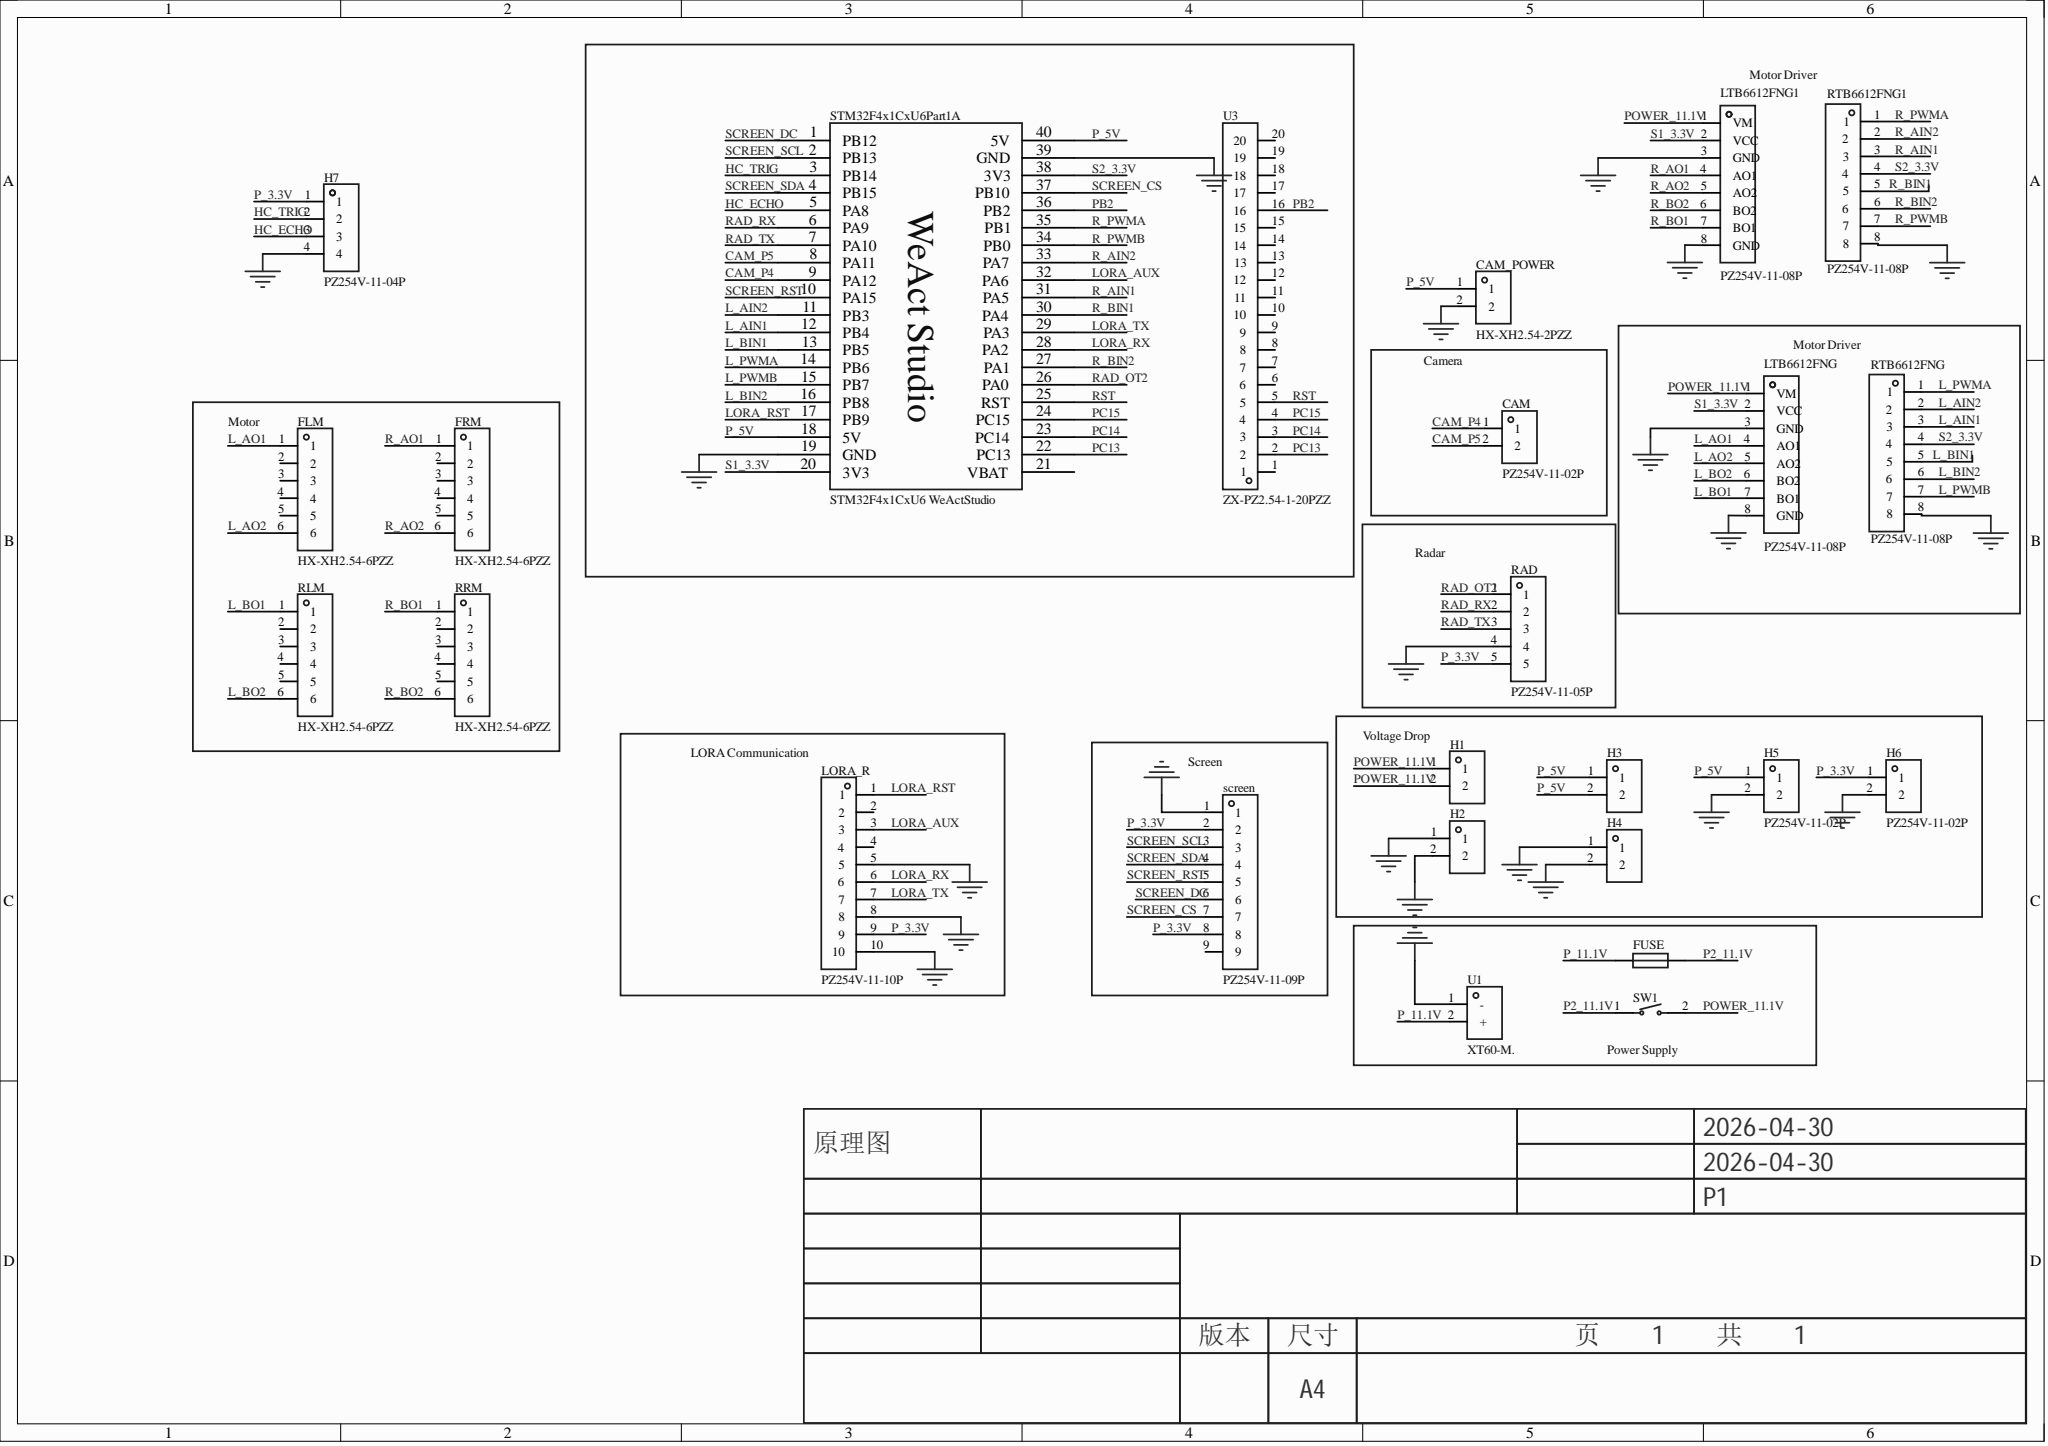Circuit board | Altium Designer | 25 parts | 49 nets
Bill of materials:
Comment,Description,Designator,Footprint,LibRef,Quantity
"PZ254V-11-02P","插针结构:1x2P;间距:2.54mm;行距:-;圆针/方针:方针;安装方式:直插;排数:单排;总PIN位数:2P;额定电流:3A;额定电压:250V;配合针长度:6mm;塑高:2.5mm;端接针长度:3mm;触头材质:黄铜;触头镀层:-;工作温度:-40℃~+105℃;颜色:黑色;","CAM, H1, H2, H3, H4, H5, H6","HDR-TH_2P-P2.54-V-M","PZ254V-11-02P","7"
"HX-XH2.54-2PZZ","插针结构:1x2P;间距:2.54mm;安装方式:直插;参考系列:XH;总PIN数:2P;排数:1;每排PIN数:2;行距:-;额定电流:3A;触头材质:黄铜;触头镀层:锡;工作温度:-25℃~+85℃;","CAM_POWER","CONN-TH_2P-P2.50_HX-2.54MM-2P-ZZ-MS","HX-XH2.54-2PZZ","1"
"HX-XH2.54-6PZZ","插针结构:1x6P;间距:2.54mm;安装方式:直插;参考系列:XH;总PIN数:6P;排数:1;每排PIN数:6;行距:-;额定电流:3A;触头材质:黄铜;触头镀层:锡;工作温度:-25℃~+85℃;","FLM, FRM, RLM, RRM","CONN-TH_6P-P2.50_BX-XH2.54-6PZZ","HX-XH2.54-6PZZ","4"
"","类型:贴片式保险丝;额定电流:3A;额定电压:32V;分断能力:50A@32VDC;","FUSE","F1206","QF1206F3A00T","1"
"PZ254V-11-04P","插针结构:1x4P;间距:2.54mm;行距:-;圆针/方针:方针;安装方式:直插;排数:单排;总PIN位数:4P;额定电流:3A;额定电压:250V;配合针长度:6mm;塑高:2.5mm;端接针长度:3mm;触头材质:-;工作温度:-40℃~+105℃;颜色:黑色;","H7","HDR-TH_4P-P2.54-V-M","PZ254V-11-04P","1"
"PZ254V-11-10P","插针结构:1x10P;间距:2.54mm;行距:-;圆针/方针:方针;安装方式:直插;排数:单排;总PIN位数:10P;额定电流:3A;额定电压:250V;配合针长度:6mm;塑高:2.5mm;端接针长度:3mm;触头材质:黄铜;触头镀层:-;工作温度:-40℃~+105℃;颜色:黑色;","LORA_R","HDR-TH_10P-P2.54-V-M","PZ254V-11-10P","1"
"PZ254V-11-08P","插针结构:1x8P;间距:2.54mm;行距:-;圆针/方针:方针;安装方式:直插;排数:单排;总PIN位数:8P;额定电流:3A;额定电压:250V;配合针长度:6mm;塑高:2.5mm;端接针长度:3mm;触头材质:黄铜;触头镀层:-;工作温度:-40℃~+105℃;颜色:黑色;","LTB6612FNG, LTB6612FNG1, RTB6612FNG, RTB6612FNG1","HDR-TH_8P-P2.54-V-M","PZ254V-11-08P","4"
"PZ254V-11-05P","插针结构:1x5P;间距:2.54mm;行距:-;圆针/方针:方针;安装方式:直插;排数:单排;总PIN位数:5P;额定电流:3A;额定电压:250V;配合针长度:6mm;塑高:2.5mm;端接针长度:3mm;触头材质:黄铜;触头镀层:-;工作温度:-40℃~+105℃;颜色:黑色;","RAD","HDR-TH_5P-P2.54-V-M","PZ254V-11-05P","1"
"PZ254V-11-09P","插针结构:1x9P;间距:2.54mm;行距:-;圆针/方针:方针;安装方式:直插;排数:单排;总PIN位数:9P;额定电流:3A;额定电压:250V;配合针长度:6mm;塑高:2.5mm;端接针长度:3mm;触头材质:黄铜;触头镀层:-;工作温度:-40℃~+105℃;颜色:黑色;","screen","HDR-TH_9P-P2.54-V-M","PZ254V-11-09P","1"
"STM32F4x1CxU6 WeActStudio","STM32F4x1CxU6","STM32F4x1CxU6Part1","STM32F4x1CxU6 WeActStudio","STM32F4x1CxU6 WeActStudio","1"
"HX KCD11-BL","带灯:无;引脚样式:焊片;额定电流:3A;额定电压(AC):250V;电路结构:单刀单掷;工作寿命:1万次;","SW1","SW-TH_KCD11-BL","HX KCD11-BL","1"
"XT60-M.","模型锂电连接器 XT60-M","U1","CONN-TH_XT60","XT60-M.","1"
"ZX-PZ2.54-1-20PZZ","插针结构:1x20P;间距:2.54mm;行距:-;圆针/方针:方针;安装方式:直插;排数:单排;总PIN位数:20P;额定电流:3A;额定电压:-;配合针长度:6mm;塑高:2.5mm;端接针长度:3mm;触头材质:黄铜;触头镀层:金;工作温度:-40℃~+105℃;颜色:黑色;","U3","HDR-TH_20P-P2.54-V-M","ZX-PZ2.54-1-20PZZ","1"
Netlist (Protel format):
[
CAM
HDR-TH_2P-P2.54-V-M
PZ254V-11-02P



]
[
CAM_POWER
CONN-TH_2P-P2.50_HX-2.54MM-2P-ZZ-MS
HX-XH2.54-2PZZ



]
[
FLM
CONN-TH_6P-P2.50_BX-XH2.54-6PZZ
HX-XH2.54-6PZZ



]
[
FRM
CONN-TH_6P-P2.50_BX-XH2.54-6PZZ
HX-XH2.54-6PZZ



]
[
FUSE
F1206




]
[
H1
HDR-TH_2P-P2.54-V-M
PZ254V-11-02P



]
[
H2
HDR-TH_2P-P2.54-V-M
PZ254V-11-02P



]
[
H3
HDR-TH_2P-P2.54-V-M
PZ254V-11-02P



]
[
H4
HDR-TH_2P-P2.54-V-M
PZ254V-11-02P



]
[
H5
HDR-TH_2P-P2.54-V-M
PZ254V-11-02P



]
[
H6
HDR-TH_2P-P2.54-V-M
PZ254V-11-02P



]
[
H7
HDR-TH_4P-P2.54-V-M
PZ254V-11-04P



]
[
LORA_R
HDR-TH_10P-P2.54-V-M
PZ254V-11-10P



]
[
LTB6612FNG
HDR-TH_8P-P2.54-V-M
PZ254V-11-08P



]
[
LTB6612FNG1
HDR-TH_8P-P2.54-V-M
PZ254V-11-08P



]
[
RAD
HDR-TH_5P-P2.54-V-M
PZ254V-11-05P



]
[
RLM
CONN-TH_6P-P2.50_BX-XH2.54-6PZZ
HX-XH2.54-6PZZ



]
[
RRM
CONN-TH_6P-P2.50_BX-XH2.54-6PZZ
HX-XH2.54-6PZZ



]
[
RTB6612FNG
HDR-TH_8P-P2.54-V-M
PZ254V-11-08P



]
[
RTB6612FNG1
HDR-TH_8P-P2.54-V-M
PZ254V-11-08P



]
[
screen
HDR-TH_9P-P2.54-V-M
PZ254V-11-09P



]
[
STM32F4x1CxU6Part1
STM32F4x1CxU6 WeActStudio
STM32F4x1CxU6 WeActStudio



]
[
SW1
SW-TH_KCD11-BL
HX KCD11-BL



]
[
U1
CONN-TH_XT60
XT60-M.



]
[
U3
HDR-TH_20P-P2.54-V-M
ZX-PZ2.54-1-20PZZ



]
(
SCREEN_SDA
screen-4
STM32F4x1CxU6Part1-4
)
(
SCREEN_SCL
screen-3
STM32F4x1CxU6Part1-2
)
(
SCREEN_RST
screen-5
STM32F4x1CxU6Part1-10
)
(
SCREEN_DC
screen-6
STM32F4x1CxU6Part1-1
)
(
SCREEN_CS
screen-7
STM32F4x1CxU6Part1-37
)
(
S2_3.3V
RTB6612FNG-4
RTB6612FNG1-4
STM32F4x1CxU6Part1-38
)
(
S1_3.3V
LTB6612FNG-2
LTB6612FNG1-2
STM32F4x1CxU6Part1-20
)
(
RST
STM32F4x1CxU6Part1-25
U3-5
)
(
RAD_TX
RAD-3
STM32F4x1CxU6Part1-7
)
(
RAD_RX
RAD-2
STM32F4x1CxU6Part1-6
)
(
RAD_OT2
RAD-1
STM32F4x1CxU6Part1-26
)
(
R_PWMB
RTB6612FNG1-7
STM32F4x1CxU6Part1-34
)
(
R_PWMA
RTB6612FNG1-1
STM32F4x1CxU6Part1-35
)
(
R_BO2
LTB6612FNG1-6
RRM-6
)
(
R_BO1
LTB6612FNG1-7
RRM-1
)
(
R_BIN2
RTB6612FNG1-6
STM32F4x1CxU6Part1-27
)
(
R_BIN1
RTB6612FNG1-5
STM32F4x1CxU6Part1-30
)
(
R_AO2
FRM-6
LTB6612FNG1-5
)
(
R_AO1
FRM-1
LTB6612FNG1-4
)
(
R_AIN2
RTB6612FNG1-2
STM32F4x1CxU6Part1-33
)
(
R_AIN1
RTB6612FNG1-3
STM32F4x1CxU6Part1-31
)
(
POWER_11.1V
H1-1
H1-2
LTB6612FNG-1
LTB6612FNG1-1
SW1-2
)
(
PC15
STM32F4x1CxU6Part1-24
U3-4
)
(
PC14
STM32F4x1CxU6Part1-23
U3-3
)
(
PC13
STM32F4x1CxU6Part1-22
U3-2
)
(
PB2
STM32F4x1CxU6Part1-36
U3-16
)
(
P_11.1V
FUSE-1
U1-2
)
(
P_5V
CAM_POWER-1
H3-1
H3-2
H5-1
STM32F4x1CxU6Part1-18
STM32F4x1CxU6Part1-40
)
(
P_3.3V
H6-1
H7-1
LORA_R-9
RAD-5
screen-2
screen-8
)
(
P2_11.1V
FUSE-2
SW1-1
)
(
LORA_TX
LORA_R-7
STM32F4x1CxU6Part1-29
)
(
LORA_RX
LORA_R-6
STM32F4x1CxU6Part1-28
)
(
LORA_RST
LORA_R-1
STM32F4x1CxU6Part1-17
)
(
LORA_AUX
LORA_R-3
STM32F4x1CxU6Part1-32
)
(
L_PWMB
RTB6612FNG-7
STM32F4x1CxU6Part1-15
)
(
L_PWMA
RTB6612FNG-1
STM32F4x1CxU6Part1-14
)
(
L_BO2
LTB6612FNG-6
RLM-6
)
(
L_BO1
LTB6612FNG-7
RLM-1
)
(
L_BIN2
RTB6612FNG-6
STM32F4x1CxU6Part1-16
)
(
L_BIN1
RTB6612FNG-5
STM32F4x1CxU6Part1-13
)
(
L_AO2
FLM-6
LTB6612FNG-5
)
(
L_AO1
FLM-1
LTB6612FNG-4
)
(
L_AIN2
RTB6612FNG-2
STM32F4x1CxU6Part1-11
)
(
L_AIN1
RTB6612FNG-3
STM32F4x1CxU6Part1-12
)
(
HC_TRIG
H7-2
STM32F4x1CxU6Part1-3
)
(
HC_ECHO
H7-3
STM32F4x1CxU6Part1-5
)
(
GND
CAM_POWER-2
H2-1
H2-2
H4-1
H4-2
H5-2
H6-2
H7-4
LORA_R-5
LORA_R-8
LORA_R-10
LTB6612FNG-3
LTB6612FNG-8
LTB6612FNG1-3
LTB6612FNG1-8
RAD-4
RTB6612FNG-8
RTB6612FNG1-8
screen-1
STM32F4x1CxU6Part1-19
STM32F4x1CxU6Part1-39
U1-1
)
(
CAM_P5
CAM-2
STM32F4x1CxU6Part1-8
)
(
CAM_P4
CAM-1
STM32F4x1CxU6Part1-9
)